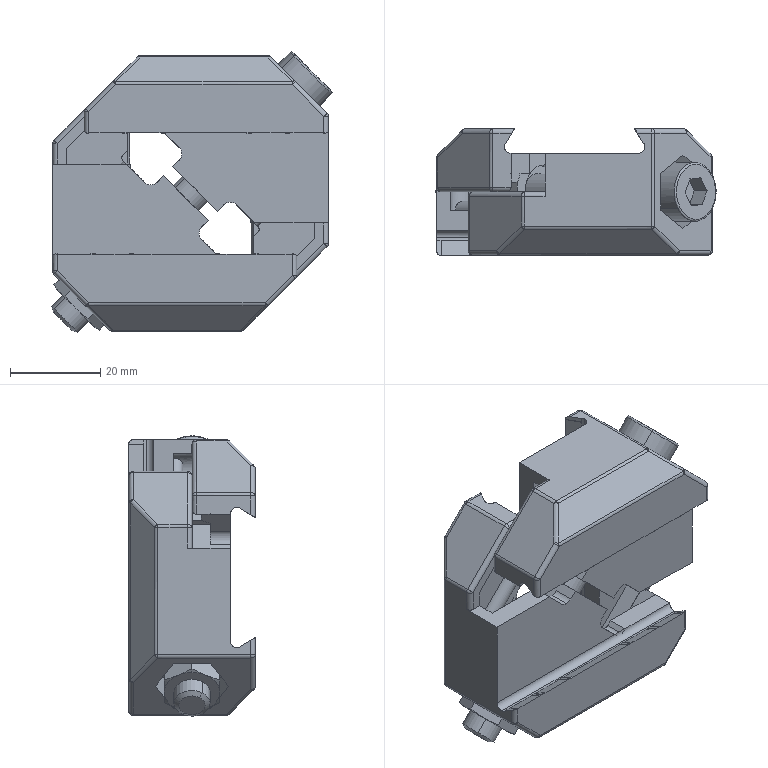Part | STEP file | 46A-01010CC13 | 6 solids | 626 faces | box 61.971 x 28 x 61.971 mm | volume 69920 mm3 | plane 391 | cylinder 165 | other 66 | spline 4 | commonest cylinder face diameters 2 x90 4 x30 8 x13 3 x12 8.2 x6 12 x6